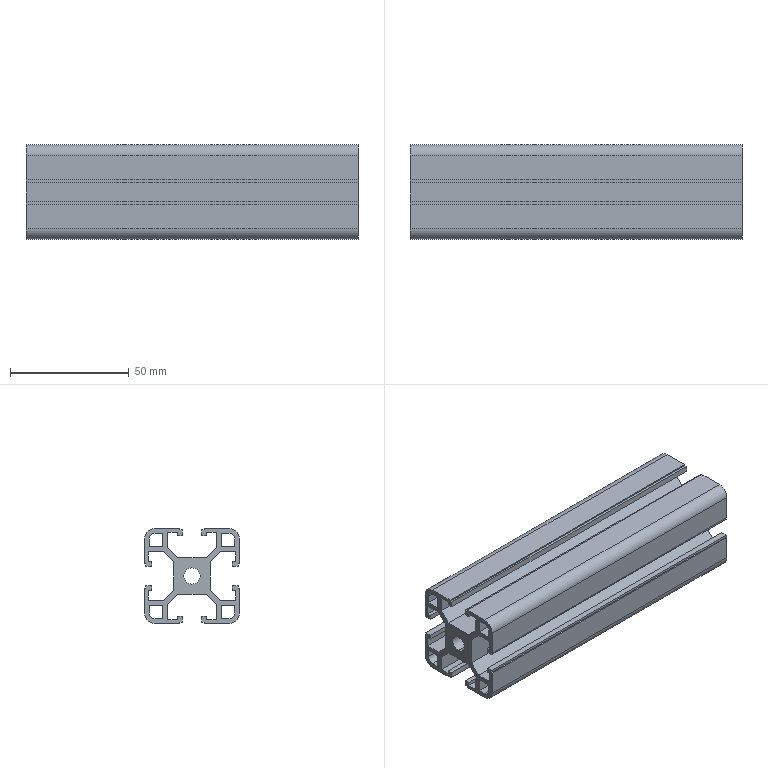Part | SolidWorks | features WeldMemberFeat 1, WeldmentFeature 1 | 1 solid | 104 faces | box 140 x 40 x 40 mm | volume 80716 mm3 | plane 94 | cylinder 10 | commonest cylinder face diameters 5 x4 9 x4 6.8 x2